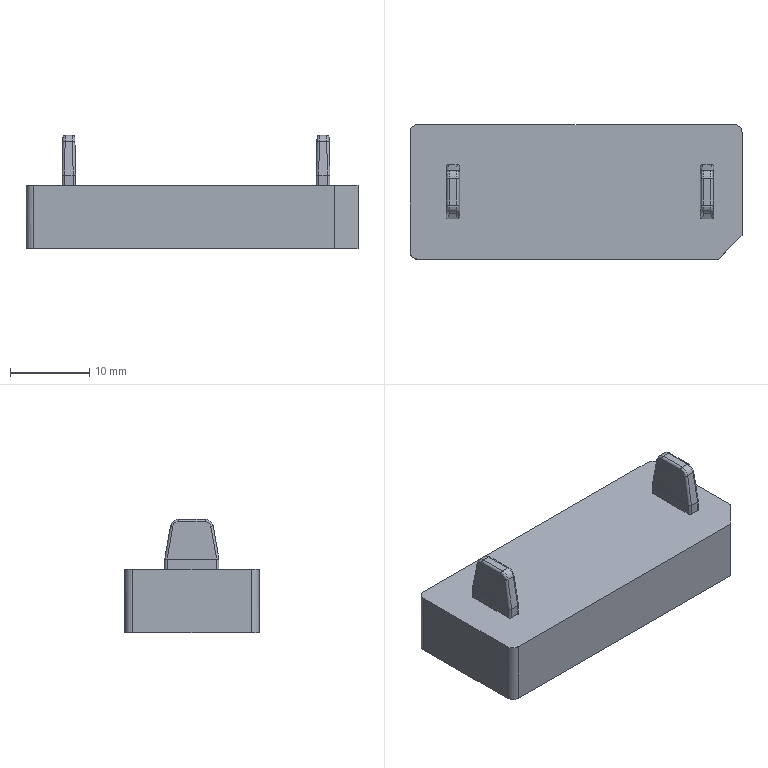NC program | PowerMill | posted by the shop | part box 42 x 17 x 14.346 mm
Lines 19164 to 20582 of 50900:
( TOOL ID   B4R0.5_2_1 )
( TOOL DIA. 4. TIP RAD .5 LENGTH 61.4 )
( Z = -6.519 )
T5 M6
T13
G91 G28 Z0
G0 G90 G54
M08
S18000 M3
X0 Y0 M8
G43 Z10.796 H5
X18.245 Y-3.811
Z.801
G1 Z-.399 F1200
X18.223 Y-3.743 F2000
X18.195 Y-3.678
X18.159 Y-3.616
X18.117 Y-3.558
X18.068 Y-3.506
X18.014 Y-3.459
X17.955 Y-3.419
X17.892 Y-3.386
X17.825 Y-3.359
X17.756 Y-3.341
X17.686 Y-3.33
X17.614 Y-3.327
X17.543 Y-3.332
X17.473 Y-3.345
X17.468 Y-3.346
X17.366 Y-3.372
X17.287 Y-3.386
X17.207 Y-3.398
X17.126 Y-3.404
X17.045 Y-3.406
X16.965
X16.575 Y-3.405
X16.186 Y-3.407
X16.072 Y-3.406
X15.958 Y-3.397
X15.845 Y-3.381
X15.733 Y-3.357
X15.623 Y-3.325
X15.516 Y-3.286
X15.412 Y-3.239
X15.321 Y-3.19
X15.232 Y-3.134
X15.142 Y-3.069
X15.05 Y-2.992
X14.972 Y-2.919
X14.899 Y-2.84
X14.83 Y-2.755
X14.766 Y-2.662
X14.706 Y-2.563
X14.652 Y-2.456
X14.603 Y-2.344
X14.56 Y-2.224
X14.536 Y-2.144
X14.518 Y-2.062
X14.502 Y-1.962
X14.489 Y-1.835
X14.481 Y-1.716
X14.478 Y-1.622
Y-1.538
X14.48 Y-.072
X14.481 Y.907
X14.479 Y1.531
X14.478 Y1.626
X14.479 Y1.722
X14.483 Y1.817
X14.49 Y1.913
X14.503 Y2.017
X14.524 Y2.125
X14.548 Y2.221
X14.577 Y2.312
X14.609 Y2.402
X14.653 Y2.503
X14.705 Y2.603
X14.765 Y2.701
X14.833 Y2.798
X14.902 Y2.884
X14.978 Y2.965
X15.061 Y3.043
X15.15 Y3.115
X15.244 Y3.181
X15.342 Y3.24
X15.444 Y3.293
X15.55 Y3.338
X15.658 Y3.376
X15.759 Y3.404
X15.865 Y3.425
X15.977 Y3.438
X16.096 Y3.445
X16.221 Y3.446
X17.104 Y3.443
X17.153 Y3.442
X17.203 Y3.438
X17.255 Y3.431
X17.323 Y3.419
X17.419 Y3.398
X17.495 Y3.378
X17.551 Y3.36
X17.598 Y3.343
X17.71 Y3.296
X17.807 Y3.248
X17.892 Y3.197
X17.973 Y3.142
X18.067 Y3.068
X18.154 Y2.99
X18.235 Y2.908
X18.308 Y2.822
X18.374 Y2.732
X18.433 Y2.639
X18.486 Y2.542
X18.538 Y2.43
X18.582 Y2.318
X18.618 Y2.205
X18.646 Y2.092
X18.663 Y1.991
X18.675 Y1.884
X18.681 Y1.759
Y1.599
X18.679 Y1.253
X18.68 Y.451
Y-.617
Y-1.551
X18.678 Y-1.721
X18.672 Y-1.851
X18.66 Y-1.963
X18.643 Y-2.064
X18.618 Y-2.164
X18.584 Y-2.27
X18.548 Y-2.367
X18.514 Y-2.448
X18.473 Y-2.527
X18.424 Y-2.613
X18.36 Y-2.71
X18.289 Y-2.805
X18.221 Y-2.885
X18.158 Y-2.951
X18.093 Y-3.01
X18.001 Y-3.084
X17.905 Y-3.15
X17.806 Y-3.208
X17.705 Y-3.259
X17.601 Y-3.303
X17.496 Y-3.338
X17.468 Y-3.346
X17.366 Y-3.373 Z-.4
X17.292 Y-3.387
X17.21 Y-3.4
X17.129 Y-3.407
X17.046 Y-3.41
X16.964
X16.5 Y-3.415 Z-.401
X16.159 Y-3.419 Z-.402
X16.036 Y-3.417
X15.923 Y-3.408 Z-.403
X15.817 Y-3.393
X15.717 Y-3.37
X15.62 Y-3.341
X15.506 Y-3.3
X15.404 Y-3.256
X15.325 Y-3.215 Z-.404
X15.248 Y-3.171
X15.175 Y-3.121
X15.099 Y-3.062
X15.032 Y-3.004
X14.967 Y-2.943 Z-.405
X14.905 Y-2.88
X14.836 Y-2.799
X14.769 Y-2.71
X14.707 Y-2.613 Z-.406
X14.65 Y-2.51
X14.601 Y-2.404
X14.56 Y-2.302 Z-.407
X14.525 Y-2.197
X14.495 Y-2.088
X14.474 Y-1.978 Z-.408
X14.46 Y-1.87
X14.453 Y-1.761
X14.45 Y-1.652 Z-.409
X14.443 Y-1.026 Z-.41
X14.437 Y-.195 Z-.413
X14.432 Y.722 Z-.415
X14.426 Y1.48 Z-.417
X14.425 Y1.605
Y1.732 Z-.418
X14.43 Y1.869
X14.44 Y1.986
X14.456 Y2.091 Z-.419
X14.478 Y2.195
X14.507 Y2.298
X14.546 Y2.411
X14.592 Y2.521
X14.646 Y2.63
X14.708 Y2.735
X14.777 Y2.837
X14.847 Y2.928
X14.924 Y3.014
X15.007 Y3.096 Z-.42
X15.097 Y3.173
X15.187 Y3.241
X15.282 Y3.302
X15.383 Y3.358
X15.489 Y3.408
X15.6 Y3.451 Z-.421
X15.703 Y3.484
X15.809 Y3.51
X15.92 Y3.528
X16.036 Y3.54 Z-.422
X16.156 Y3.544
X16.264
X16.515 Y3.545 Z-.423
X16.766 Y3.547 Z-.424
X17.017 Y3.548
X17.137 Y3.549 Z-.425
X17.223 Y3.545
X17.314 Y3.533
X17.411 Y3.513
X17.517 Y3.483 Z-.426
X17.619 Y3.448
X17.727 Y3.405 Z-.427
X17.829 Y3.355
X17.926 Y3.301
X18.016 Y3.24 Z-.428
X18.102 Y3.175
X18.184 Y3.104
X18.263 Y3.028 Z-.429
X18.337 Y2.947
X18.407 Y2.858 Z-.43
X18.471 Y2.766
X18.528 Y2.669 Z-.431
X18.581 Y2.57
X18.624 Y2.474
X18.663 Y2.369 Z-.432
X18.698 Y2.255
X18.728 Y2.131
X18.751 Y2.001
X18.765 Y1.877 Z-.433
X18.772 Y1.761
X18.773 Y1.652
X18.781 Y-.205 Z-.438
X18.79 Y-1.402 Z-.441
X18.792 Y-1.554
X18.79 Y-1.713 Z-.442
X18.781 Y-1.86
X18.765 Y-1.997
X18.744 Y-2.125 Z-.443
X18.715 Y-2.245
X18.681 Y-2.359
X18.641 Y-2.467
X18.599 Y-2.56 Z-.444
X18.549 Y-2.656
X18.488 Y-2.76
X18.417 Y-2.865 Z-.445
X18.345 Y-2.959
X18.275 Y-3.04
X18.204 Y-3.111
X18.129 Y-3.177 Z-.446
X18.035 Y-3.252
X17.938 Y-3.318
X17.839 Y-3.377
X17.736 Y-3.428 Z-.447
X17.631 Y-3.472
X17.523 Y-3.51
X17.517 Y-3.512
X17.393 Y-3.544
X17.27 Y-3.567 Z-.448
X17.149 Y-3.582
X17.031 Y-3.59
X16.912 Z-.449
X16.504 Y-3.591
X16.159 Y-3.595 Z-.45
X16.055 Y-3.594 Z-.451
X15.951 Y-3.587
X15.846 Y-3.573
X15.737 Y-3.55
X15.632 Y-3.521 Z-.452
X15.531 Y-3.488
X15.424 Y-3.445
X15.324 Y-3.397
X15.23 Y-3.344 Z-.453
X15.142 Y-3.285
X15.056 Y-3.222
X14.969 Y-3.149
X14.892 Y-3.076 Z-.454
X14.82 Y-2.998
X14.753 Y-2.917
X14.681 Y-2.817
X14.615 Y-2.713 Z-.455
X14.556 Y-2.606
X14.505 Y-2.494
X14.46 Y-2.38 Z-.456
X14.423 Y-2.263
X14.391 Y-2.137
X14.367 Y-2.011 Z-.457
X14.351 Y-1.886
X14.343 Y-1.761
X14.342 Y-1.637
X14.337 Y-.269 Z-.461
X14.333 Y.812 Z-.463
X14.327 Y1.545 Z-.465
X14.326 Y1.649
X14.327 Y1.752
X14.331 Y1.856 Z-.466
X14.34 Y1.959
X14.354 Y2.07
X14.373 Y2.172
X14.397 Y2.272 Z-.467
X14.424 Y2.372
X14.463 Y2.488
X14.509 Y2.601
X14.561 Y2.709 Z-.468
X14.622 Y2.817
X14.689 Y2.919
X14.76 Y3.015
X14.837 Y3.105 Z-.469
X14.907 Y3.178
X14.987 Y3.252
X15.078 Y3.327 Z-.47
X15.177 Y3.398
X15.275 Y3.459
X15.369 Y3.51
X15.46 Y3.551 Z-.471
X15.546 Y3.583
X15.63 Y3.612
X15.716 Y3.636
X15.841 Y3.665
X15.933 Y3.68 Z-.472
X16.036 Y3.688
X16.157 Y3.691
X16.316 Z-.473
X16.772 Y3.694 Z-.474
X16.977 Y3.697
X17.1 Y3.696
X17.217 Y3.687 Z-.475
X17.329 Y3.672
X17.437 Y3.649
X17.542 Y3.62
X17.658 Y3.579 Z-.476
X17.769 Y3.533
X17.874 Y3.481
X17.975 Y3.422 Z-.477
X18.071 Y3.356
X18.163 Y3.284
X18.25 Y3.206
X18.333 Y3.121 Z-.478
X18.412 Y3.029
X18.485 Y2.933
X18.553 Y2.831 Z-.479
X18.614 Y2.723
X18.669 Y2.611
X18.717 Y2.494
X18.759 Y2.373 Z-.48
X18.794 Y2.248
X18.821 Y2.119
X18.841 Y1.987 Z-.481
X18.853 Y1.852
X18.858 Y1.716
Y1.578 Z-.482
X18.862 Y.382 Z-.484
X18.865 Y-.57 Z-.487
X18.869 Y-1.524 Z-.489
Y-1.717
X18.865 Y-1.846 Z-.49
X18.853 Y-1.975
X18.833 Y-2.104
X18.805 Y-2.232
X18.769 Y-2.359 Z-.491
X18.726 Y-2.484
X18.674 Y-2.608
X18.621 Y-2.717 Z-.492
X18.561 Y-2.823
X18.494 Y-2.925
X18.42 Y-3.023 Z-.493
X18.34 Y-3.117
X18.253 Y-3.205
X18.176 Y-3.276
X18.091 Y-3.344 Z-.494
X17.994 Y-3.412
X17.891 Y-3.475
X17.788 Y-3.529
X17.689 Y-3.573 Z-.495
X17.596 Y-3.608
X17.551 Y-3.621
X17.441 Y-3.654
X17.361 Y-3.674 Z-.496
X17.281 Y-3.688
X17.168 Y-3.701
X17.045 Y-3.707
X16.908 Y-3.708 Z-.497
X16.475 Y-3.71 Z-.498
X16.159 Y-3.713
X16.042 Y-3.71 Z-.499
X15.923 Y-3.701
X15.807 Y-3.684
X15.753 Y-3.673
X15.699 Y-3.659
X15.642 Y-3.642
X15.568 Y-3.619 Z-.5
X15.464 Y-3.581
X15.393 Y-3.553
X15.341 Y-3.528
X15.291 Y-3.503
X15.185 Y-3.441 Z-.501
X15.084 Y-3.374
X14.989 Y-3.3
X14.9 Y-3.222
X14.817 Y-3.138 Z-.502
X14.738 Y-3.048
X14.663 Y-2.95
X14.594 Y-2.846
X14.529 Y-2.736 Z-.503
X14.471 Y-2.621
X14.421 Y-2.503
X14.378 Y-2.384 Z-.504
X14.343 Y-2.262
X14.313 Y-2.131
X14.29 Y-1.998 Z-.505
X14.276 Y-1.869
X14.27 Y-1.745
X14.269 Y-1.621
X14.265 Y-.061 Z-.509
X14.262 Y.996 Z-.511
X14.258 Y1.593 Z-.513
X14.259 Y1.757
X14.267 Y1.908
X14.281 Y2.048 Z-.514
X14.301 Y2.178
X14.329 Y2.303
X14.363 Y2.424 Z-.515
X14.406 Y2.549
X14.455 Y2.669
X14.511 Y2.784 Z-.516
X14.573 Y2.893
X14.642 Y2.999
X14.717 Y3.099
X14.797 Y3.194 Z-.517
X14.882 Y3.282
X14.973 Y3.364
X15.067 Y3.439
X15.165 Y3.507 Z-.518
X15.267 Y3.568
X15.372 Y3.621
X15.481 Y3.668 Z-.519
X15.596 Y3.709
X15.714 Y3.742
X15.833 Y3.767
X15.953 Y3.785 Z-.52
X16.075 Y3.795
X16.196 Y3.797
X16.755 Y3.798 Z-.521
X16.918 Y3.799 Z-.522
X17.065 Y3.8
X17.179 Y3.795
X17.28 Y3.784 Z-.523
X17.322 Y3.777
X17.365 Y3.768
X17.417 Y3.757
X17.499 Y3.737
X17.55 Y3.723
X17.591 Y3.711
X17.631 Y3.695 Z-.524
X17.715 Y3.662
X17.798 Y3.628
X17.879 Y3.588
X17.983 Y3.528
X18.083 Y3.462 Z-.525
X18.179 Y3.388
X18.27 Y3.308
X18.357 Y3.221
X18.439 Y3.128 Z-.526
X18.515 Y3.029
X18.585 Y2.925
X18.65 Y2.816 Z-.527
X18.707 Y2.703
X18.758 Y2.585
X18.804 Y2.456 Z-.528
X18.843 Y2.325
X18.874 Y2.194
X18.897 Y2.064
X18.911 Y1.934 Z-.529
X18.918 Y1.806
X18.919 Y1.679
X18.923 Y.67 Z-.532
X18.927 Y-.867 Z-.535
X18.928 Y-1.714 Z-.537
X18.923 Y-1.852
X18.911 Y-1.988 Z-.538
X18.892 Y-2.123
X18.864 Y-2.256
X18.829 Y-2.387 Z-.539
X18.786 Y-2.514
X18.737 Y-2.636
X18.682 Y-2.753
X18.619 Y-2.866 Z-.54
X18.551 Y-2.974
X18.476 Y-3.077
X18.404 Y-3.165 Z-.541
X18.323 Y-3.251
X18.234 Y-3.335
X18.137 Y-3.415
X18.037 Y-3.488 Z-.542
X17.935 Y-3.552
X17.834 Y-3.608
X17.735 Y-3.654
X17.638 Y-3.691 Z-.543
X17.578 Y-3.709
X17.47 Y-3.74
X17.357 Y-3.767
X17.241 Y-3.786 Z-.544
X17.13 Y-3.798
X17.019 Y-3.803
X16.908
X16.408 Y-3.804 Z-.546
X16.16 Y-3.807
X16.046 Y-3.805
X15.93 Y-3.795 Z-.547
X15.813 Y-3.777
X15.695 Y-3.751
X15.574 Y-3.716
X15.462 Y-3.677 Z-.548
X15.352 Y-3.63
X15.245 Y-3.576
X15.143 Y-3.516
X15.045 Y-3.448 Z-.549
X14.95 Y-3.373
X14.859 Y-3.292
X14.773 Y-3.203 Z-.55
X14.691 Y-3.109
X14.615 Y-3.008
X14.545 Y-2.901
X14.48 Y-2.79 Z-.551
X14.422 Y-2.673
X14.371 Y-2.553
X14.331 Y-2.438
X14.296 Y-2.318 Z-.552
X14.265 Y-2.186
X14.24 Y-2.046
X14.224 Y-1.91 Z-.553
X14.216 Y-1.783
X14.214 Y-1.658
X14.21 Y.297 Z-.558
X14.206 Y1.717 Z-.561
X14.209 Y1.862
X14.22 Y2.005
X14.239 Y2.144 Z-.562
X14.266 Y2.281
X14.299 Y2.413
X14.339 Y2.542 Z-.563
X14.387 Y2.666
X14.441 Y2.785
X14.501 Y2.9 Z-.564
X14.568 Y3.01
X14.64 Y3.114
X14.719 Y3.213
X14.802 Y3.305 Z-.565
X14.89 Y3.391
X14.983 Y3.471
X15.071 Y3.537
X15.163 Y3.599 Z-.566
X15.264 Y3.657
X15.358 Y3.706
X15.424 Y3.735
X15.491 Y3.761
X15.573 Y3.789 Z-.567
X15.678 Y3.821
X15.748 Y3.839
X15.819 Y3.854
X15.89 Y3.865
X16.011 Y3.877 Z-.568
X16.14 Y3.882
X16.279 Y3.883
X16.852 Y3.885 Z-.57
X16.977
X17.059
X17.167 Y3.882
X17.255 Y3.873
X17.336 Y3.859 Z-.571
X17.44 Y3.838
X17.543 Y3.811
X17.66 Y3.772
X17.774 Y3.726 Z-.572
X17.884 Y3.673
X17.991 Y3.614
X18.093 Y3.547
X18.191 Y3.473 Z-.573
X18.283 Y3.395
X18.369 Y3.312
X18.451 Y3.221 Z-.574
X18.529 Y3.123
X18.602 Y3.019
X18.669 Y2.909
X18.73 Y2.793 Z-.575
X18.785 Y2.673
X18.832 Y2.549
X18.873 Y2.423 Z-.576
X18.907 Y2.292
X18.933 Y2.158
X18.953 Y2.02
X18.965 Y1.879 Z-.577
X18.97 Y1.732
Y1.583
X18.972 Y.357 Z-.58
X18.974 Y-.867 Z-.583
X18.978 Y-1.582 Z-.584
X18.976 Y-1.75 Z-.585
X18.967 Y-1.907
X18.951 Y-2.054 Z-.586
X18.928 Y-2.194
X18.899 Y-2.326
X18.863 Y-2.454
X18.819 Y-2.582 Z-.587
X18.768 Y-2.705
X18.711 Y-2.824
X18.647 Y-2.937 Z-.588
X18.578 Y-3.046
X18.51 Y-3.138
X18.437 Y-3.226
X18.351 Y-3.318 Z-.589
X18.255 Y-3.41
X18.163 Y-3.489
X18.119 Y-3.523
X18.081 Y-3.55
X18.04 Y-3.576 Z-.59
X17.987 Y-3.608
X17.915 Y-3.648
X17.814 Y-3.7
X17.743 Y-3.733
X17.687 Y-3.756
X17.643 Y-3.772 Z-.591
X17.599 Y-3.784
X17.495 Y-3.815
X17.389 Y-3.841
X17.279 Y-3.86
X17.17 Y-3.872 Z-.592
X17.062 Y-3.878
X16.953 Y-3.88
X16.432 Y-3.882 Z-.593
X16.16 Y-3.883 Z-.594
X16.076
X15.994 Y-3.879
X15.9 Y-3.868
X15.832 Y-3.859 Z-.595
X15.803 Y-3.854
X15.772 Y-3.848
X15.723 Y-3.837
X15.694 Y-3.83
X15.666 Y-3.823
X15.566 Y-3.794
X15.488 Y-3.769
X15.375 Y-3.723 Z-.596
X15.266 Y-3.67
X15.159 Y-3.61
X15.057 Y-3.543
X14.958 Y-3.469 Z-.597
X14.864 Y-3.389
X14.775 Y-3.302
X14.692 Y-3.21 Z-.598
X14.614 Y-3.111
X14.542 Y-3.007
X14.475 Y-2.897
X14.413 Y-2.781 Z-.599
X14.359 Y-2.66
X14.31 Y-2.535
X14.268 Y-2.403 Z-.6
X14.233 Y-2.268
X14.205 Y-2.132
X14.186 Y-1.993
X14.174 Y-1.852 Z-.601
X14.17 Y-1.709
X14.168 Y-.346 Z-.604
X14.165 Y.94 Z-.607
X14.162 Y1.593 Z-.608
X14.164 Y1.775 Z-.609
X14.172 Y1.937
X14.186 Y2.084
X14.207 Y2.221 Z-.61
X14.234 Y2.351
X14.27 Y2.486
X14.313 Y2.616 Z-.611
X14.363 Y2.741
X14.42 Y2.862
X14.482 Y2.978
X14.55 Y3.087 Z-.612
X14.624 Y3.191
X14.703 Y3.288
X14.787 Y3.38 Z-.613
X14.876 Y3.465
X14.969 Y3.543
X15.067 Y3.614
X15.173 Y3.684 Z-.614
X15.276 Y3.742
X15.376 Y3.791
X15.459 Y3.825
X15.543 Y3.856
X15.63 Y3.882 Z-.615
X15.689 Y3.898
X15.748 Y3.914
X15.808 Y3.927
X15.869 Y3.935
X15.969 Y3.948
X16.053 Y3.954 Z-.616
X16.16 Y3.955
X16.739 Y3.957 Z-.617
X16.979 Y3.958 Z-.618
X17.103 Y3.955
X17.227 Y3.946
X17.35 Y3.929
X17.46 Y3.907 Z-.619
X17.549 Y3.885
X17.636 Y3.857
X17.729 Y3.821
X17.837 Y3.774 Z-.62
X17.944 Y3.72
X18.032 Y3.668
X18.108 Y3.617
X18.215 Y3.536 Z-.621
X18.307 Y3.457
X18.389 Y3.378
X18.475 Y3.284
X18.553 Y3.187 Z-.622
X18.625 Y3.084
X18.693 Y2.975
X18.754 Y2.86
X18.81 Y2.74 Z-.623
X18.859 Y2.615
X18.902 Y2.485
X18.938 Y2.351 Z-.624
X18.967 Y2.211
X18.988 Y2.067
X19.003 Y1.919 Z-.625
X19.009 Y1.768
X19.01 Y1.613
X19.014 Y-.465 Z-.63
Y-1.715 Z-.633
X19.01 Y-1.863
X18.998 Y-2.009
X18.978 Y-2.152 Z-.634
X18.951 Y-2.292
X18.917 Y-2.428
X18.876 Y-2.561
X18.827 Y-2.688 Z-.635
X18.773 Y-2.812
X18.711 Y-2.93
X18.647 Y-3.038 Z-.636
X18.577 Y-3.142
X18.499 Y-3.243
X18.413 Y-3.34
X18.328 Y-3.425 Z-.637
X18.235 Y-3.507
X18.137 Y-3.583
X18.033 Y-3.654 Z-.638
X17.927 Y-3.716
X17.818 Y-3.771
X17.709 Y-3.817
X17.618 Y-3.85 Z-.639
X17.514 Y-3.88
X17.41 Y-3.906
X17.301 Y-3.927
X17.194 Y-3.941
X17.086 Y-3.948 Z-.64
X16.979 Y-3.95
X16.871 Y-3.949
X16.336 Y-3.95 Z-.641
X16.16 Y-3.952 Z-.642
X16.039 Y-3.95
X15.917 Y-3.939
X15.796 Y-3.921
X15.674 Y-3.895 Z-.643
X15.554 Y-3.86
X15.437 Y-3.819
X15.323 Y-3.77 Z-.644
X15.213 Y-3.714
X15.107 Y-3.651
X15.007 Y-3.582
X14.911 Y-3.508 Z-.645
X14.817 Y-3.424
X14.728 Y-3.334
X14.645 Y-3.239
X14.569 Y-3.139 Z-.646
X14.499 Y-3.034
X14.432 Y-2.921
X14.371 Y-2.802 Z-.647
X14.317 Y-2.679
X14.27 Y-2.551
X14.229 Y-2.42
X14.196 Y-2.285 Z-.648
X14.17 Y-2.148
X14.15 Y-2.
X14.138 Y-1.853 Z-.649
X14.134 Y-1.707
X14.131 Y-.191 Z-.652
X14.13 Y1.064 Z-.655
X14.127 Y1.593 Z-.656
X14.128 Y1.723
X14.131 Y1.854 Z-.657
X14.139 Y1.984
X14.155 Y2.122
X14.175 Y2.251
X14.201 Y2.376 Z-.658
X14.235 Y2.511
X14.276 Y2.64
X14.323 Y2.761 Z-.659
X14.376 Y2.878
X14.439 Y2.998
X14.507 Y3.111
X14.579 Y3.217 Z-.66
X14.657 Y3.315
X14.738 Y3.407
X14.827 Y3.496 Z-.661
X14.922 Y3.579
X15.019 Y3.655
X15.117 Y3.721
X15.215 Y3.779 Z-.662
X15.299 Y3.824
X15.386 Y3.863
X15.479 Y3.9
X15.59 Y3.937
X15.686 Y3.963 Z-.663
X15.766 Y3.98
X15.87 Y4.
X15.949 Y4.011
X16.021 Y4.014
X16.365 Y4.019 Z-.664
X16.704 Y4.02 Z-.665
X16.892 Y4.022
X17.05 Y4.021 Z-.666
X17.176 Y4.015
X17.285 Y4.004
X17.391 Y3.986
X17.513 Y3.958 Z-.667
X17.633 Y3.923
X17.748 Y3.881
X17.86 Y3.831
X17.968 Y3.775 Z-.668
X18.073 Y3.711
X18.174 Y3.641
X18.271 Y3.563
X18.364 Y3.479 Z-.669
X18.451 Y3.389
X18.533 Y3.294
X18.61 Y3.193 Z-.67
X18.681 Y3.087
X18.746 Y2.975
X18.805 Y2.857
X18.859 Y2.734 Z-.671
X18.905 Y2.605
X18.946 Y2.472
X18.98 Y2.333 Z-.672
X19.006 Y2.189
X19.026 Y2.04
X19.038 Y1.887 Z-.673
X19.043 Y1.73
Y1.57
X19.044 Y.166 Z-.676
X19.046 Y-1.582 Z-.68
Y-1.695
X19.043 Y-1.807 Z-.681
X19.038 Y-1.92
X19.029 Y-2.032
X19.014 Y-2.144
X18.992 Y-2.265 Z-.682
X18.967 Y-2.375
X18.938 Y-2.484
X18.905 Y-2.591
X18.86 Y-2.717 Z-.683
X18.807 Y-2.839
X18.748 Y-2.956
X18.682 Y-3.069
X18.611 Y-3.176 Z-.684
X18.533 Y-3.278
X18.45 Y-3.375
X18.36 Y-3.466
X18.266 Y-3.551 Z-.685
X18.168 Y-3.629
X18.065 Y-3.7
X17.96 Y-3.764 Z-.686
X17.851 Y-3.82
X17.741 Y-3.868
X17.639 Y-3.905
X17.574 Y-3.926
X17.509 Y-3.944 Z-.687
X17.422 Y-3.966
X17.317 Y-3.987
X17.239 Y-3.998
X17.172 Y-4.005
X17.104 Y-4.007
X16.603 Y-4.012 Z-.689
X16.251
X15.996 Y-4.007 Z-.69
X15.905 Y-4.
X15.807 Y-3.985
X15.698 Y-3.962
X15.573 Y-3.927 Z-.691
X15.469 Y-3.893
X15.366 Y-3.853
X15.262 Y-3.804
X15.156 Y-3.746 Z-.692
X15.048 Y-3.678
X14.949 Y-3.607
X14.855 Y-3.529 Z-.693
X14.764 Y-3.444
X14.678 Y-3.353
X14.597 Y-3.255
X14.521 Y-3.15 Z-.694
X14.45 Y-3.04
X14.385 Y-2.925
X14.327 Y-2.804
X14.275 Y-2.679 Z-.695
X14.23 Y-2.549
X14.192 Y-2.414
X14.16 Y-2.273 Z-.696
X14.135 Y-2.127
X14.117 Y-1.978
X14.107 Y-1.825 Z-.697
X14.105 Y-1.67
X14.101 Y.341 Z-.701
X14.099 Y1.714 Z-.704
X14.102 Y1.856
X14.112 Y2.01 Z-.705
X14.13 Y2.167
X14.155 Y2.315
X14.184 Y2.45 Z-.706
X14.218 Y2.575
X14.262 Y2.706
X14.312 Y2.833 Z-.707
X14.368 Y2.954
X14.431 Y3.07
X14.5 Y3.181
X14.575 Y3.286 Z-.708
X14.656 Y3.386
X14.742 Y3.481
X14.834 Y3.57
X14.926 Y3.648 Z-.709
X15.023 Y3.722
X15.128 Y3.79
X15.218 Y3.842
X15.31 Y3.889 Z-.71
X15.405 Y3.931
X15.502 Y3.967
X15.596 Y3.998
X15.712 Y4.03 Z-.711
X15.823 Y4.052
X15.926 Y4.066
X16.024 Y4.072
X16.212 Y4.076 Z-.712
X16.399
X16.587
X16.978 Y4.077 Z-.713
X17.11 Y4.075 Z-.714
X17.238 Y4.065
X17.362 Y4.048
X17.483 Y4.023
X17.602 Y3.991 Z-.715
X17.718 Y3.951
X17.831 Y3.904
X17.94 Y3.85
X18.046 Y3.789 Z-.716
X18.15 Y3.72
X18.251 Y3.643
X18.349 Y3.559
X18.44 Y3.469 Z-.717
X18.525 Y3.376
X18.601 Y3.28
X18.675 Y3.174 Z-.718
X18.743 Y3.063
X18.805 Y2.947
X18.861 Y2.826
X18.91 Y2.699 Z-.719
X18.953 Y2.566
X18.99 Y2.428
X19.02 Y2.284 Z-.72
X19.043 Y2.135
X19.059 Y1.98
X19.068 Y1.82 Z-.721
X19.07 Y1.654
X19.072 Y-.697 Z-.726
X19.073 Y-1.717 Z-.728
X19.069 Y-1.873
X19.057 Y-2.027 Z-.729
X19.038 Y-2.177
X19.011 Y-2.325
X18.977 Y-2.469 Z-.73
X18.935 Y-2.609
X18.891 Y-2.735
X18.839 Y-2.858 Z-.731
X18.781 Y-2.977
X18.715 Y-3.092
X18.643 Y-3.202
X18.565 Y-3.307 Z-.732
X18.481 Y-3.408
X18.397 Y-3.496
X18.307 Y-3.579 Z-.733
X18.21 Y-3.659
X18.107 Y-3.732
X18.001 Y-3.798
X17.893 Y-3.856 Z-.734
X17.785 Y-3.906
X17.678 Y-3.947
X17.657 Y-3.954
X17.59 Y-3.978
X17.511 Y-4.
X17.406 Y-4.023 Z-.735
X17.297 Y-4.043
X17.212 Y-4.055
X17.113 Y-4.061
X16.982 Y-4.063 Z-.736
X16.446 Y-4.064 Z-.737
X16.158 Y-4.065
X16.032 Y-4.062 Z-.738
X15.906 Y-4.051
X15.78 Y-4.032
X15.656 Y-4.005
X15.537 Y-3.972 Z-.739
X15.421 Y-3.931
X15.307 Y-3.882
X15.197 Y-3.827
X15.09 Y-3.764 Z-.74
X14.987 Y-3.694
X14.888 Y-3.618
X14.793 Y-3.535
X14.703 Y-3.445 Z-.741
X14.618 Y-3.349
X14.539 Y-3.247
X14.465 Y-3.14 Z-.742
X14.398 Y-3.027
X14.337 Y-2.91
X14.28 Y-2.785
X14.231 Y-2.656 Z-.743
X14.188 Y-2.523
X14.153 Y-2.385
X14.124 Y-2.242 Z-.744
X14.102 Y-2.094
X14.087 Y-1.941
X14.08 Y-1.783 Z-.745
X14.079 Y-1.62
X14.078 Y.52 Z-.749
X14.075 Y1.593 Z-.752
X14.077 Y1.792
X14.086 Y1.969
X14.1 Y2.132 Z-.753
X14.121 Y2.282
X14.148 Y2.423
X14.18 Y2.556 Z-.754
X14.22 Y2.684
X14.266 Y2.808
X14.32 Y2.934 Z-.755
X14.379 Y3.052
X14.442 Y3.162
X14.509 Y3.264
X14.583 Y3.363 Z-.756
X14.667 Y3.463
X14.752 Y3.554
X14.839 Y3.636
X14.927 Y3.709 Z-.757
X15.019 Y3.775
X15.13 Y3.847
X15.24 Y3.909
X15.349 Y3.963 Z-.758
X15.413 Y3.99
X15.478 Y4.013
X15.543 Y4.034
X15.621 Y4.056
X15.727 Y4.083
X15.826 Y4.103 Z-.759
X15.902 Y4.115
X15.97 Y4.122
X16.039 Y4.124
X16.423 Y4.128 Z-.76
X16.704 Z-.761
X16.901 Y4.13
X17.062 Y4.129
X17.19 Y4.123 Z-.762
X17.305 Y4.111
X17.38 Y4.098
X17.455 Y4.081
X17.539 Y4.06
X17.637 Y4.032 Z-.763
X17.709 Y4.008
X17.78 Y3.981
X17.895 Y3.927
X18.008 Y3.866
X18.11 Y3.805 Z-.764
X18.202 Y3.742
X18.293 Y3.669
X18.383 Y3.588
X18.472 Y3.498 Z-.765
X18.559 Y3.398
X18.635 Y3.3
X18.706 Y3.197
X18.772 Y3.086 Z-.766
X18.832 Y2.969
X18.888 Y2.845
X18.937 Y2.717 Z-.767
X18.979 Y2.585
X19.014 Y2.448
X19.043 Y2.304
X19.065 Y2.154 Z-.768
X19.081 Y1.995
X19.09 Y1.829
X19.091 Y1.654 Z-.769
X19.093 Y-1.032 Z-.774
Y-1.714 Z-.776
X19.09 Y-1.871
X19.078 Y-2.031 Z-.777
X19.06 Y-2.188
X19.034 Y-2.339
X19.003 Y-2.481 Z-.778
X18.966 Y-2.613
X18.923 Y-2.738
X18.872 Y-2.865
X18.814 Y-2.987 Z-.779
X18.75 Y-3.103
X18.68 Y-3.215
X18.605 Y-3.32 Z-.78
X18.523 Y-3.42
X18.437 Y-3.514
X18.345 Y-3.601
X18.249 Y-3.683 Z-.781
X18.147 Y-3.758
X18.041 Y-3.828
X17.937 Y-3.886
X17.828 Y-3.939 Z-.782
X17.713 Y-3.986
X17.673 Y-4.
X17.581 Y-4.029
X17.488 Y-4.055
X17.394 Y-4.075 Z-.783
X17.269 Y-4.094
X17.14 Y-4.106
X17.002 Y-4.111
X16.857 Y-4.112 Z-.784
X16.432 Z-.785
X16.16 Y-4.113
X16.074
X15.989 Y-4.109
X15.891 Y-4.097 Z-.786
X15.83 Y-4.09
X15.769 Y-4.08
X15.709 Y-4.067
X15.623 Y-4.047
X15.563 Y-4.03
X15.504 Y-4.012 Z-.787
X15.371 Y-3.96
X15.261 Y-3.911
X15.163 Y-3.86
X15.056 Y-3.795 Z-.788
X14.953 Y-3.724
X14.854 Y-3.645
X14.76 Y-3.56
X14.67 Y-3.468 Z-.789
X14.586 Y-3.371
X14.507 Y-3.267
X14.434 Y-3.159
X14.368 Y-3.045 Z-.79
X14.308 Y-2.928
X14.255 Y-2.805
X14.208 Y-2.677 Z-.791
X14.167 Y-2.543
X14.132 Y-2.403
X14.104 Y-2.257
X14.083 Y-2.104 Z-.792
X14.069 Y-1.945
X14.062 Y-1.778
X14.061 Y-1.605 Z-.793
X14.058 Y1.032 Z-.798
Y1.716 Z-.8
X14.061 Y1.885
X14.07 Y2.049
X14.086 Y2.203 Z-.801
X14.108 Y2.348
X14.137 Y2.485
X14.172 Y2.619 Z-.802
X14.211 Y2.744
X14.256 Y2.866
X14.31 Y2.987
X14.369 Y3.103 Z-.803
X14.433 Y3.213
X14.505 Y3.321
X14.583 Y3.424
X14.667 Y3.521 Z-.804
X14.756 Y3.613
X14.851 Y3.699
X14.95 Y3.778 Z-.805
X15.054 Y3.851
X15.162 Y3.916
X15.269 Y3.972
X15.381 Y4.023 Z-.806
X15.498 Y4.066
X15.62 Y4.104
X15.745 Y4.133
X15.871 Y4.155 Z-.807
X15.996 Y4.168
X16.118 Y4.174
X16.238 Y4.173
X16.685 Z-.808
X16.976 Y4.176 Z-.809
X17.097 Y4.175
X17.223 Y4.165
X17.351 Y4.148 Z-.81
X17.478 Y4.122
X17.602 Y4.089
X17.721 Y4.05 Z-.811
X17.834 Y4.005
X17.939 Y3.954
X18.04 Y3.898
X18.146 Y3.831 Z-.812
X18.247 Y3.758
X18.342 Y3.679
X18.432 Y3.594
X18.517 Y3.504 Z-.813
X18.598 Y3.408
X18.676 Y3.303
X18.748 Y3.193
X18.813 Y3.077 Z-.814
X18.872 Y2.958
X18.924 Y2.834
X18.969 Y2.706
X19.008 Y2.573 Z-.815
X19.041 Y2.432
X19.068 Y2.284
X19.088 Y2.128 Z-.816
X19.101 Y1.962
X19.108 Y1.787
Y1.598 Z-.817
X19.11 Y-1.139 Z-.823
X19.111 Y-1.714 Z-.824
X19.107 Y-1.886
X19.096 Y-2.05
X19.077 Y-2.207 Z-.825
X19.052 Y-2.359
X19.02 Y-2.504
X18.982 Y-2.643 Z-.826
X18.937 Y-2.776
X18.888 Y-2.898
X18.833 Y-3.018 Z-.827
X18.769 Y-3.134
X18.699 Y-3.247
X18.621 Y-3.356
X18.544 Y-3.453 Z-.828
X18.458 Y-3.546
X18.366 Y-3.635
X18.269 Y-3.718
X18.167 Y-3.794 Z-.829
X18.063 Y-3.863
X17.956 Y-3.924
X17.849 Y-3.976
X17.741 Y-4.02 Z-.83
X17.687 Y-4.039
X17.604 Y-4.069
X17.519 Y-4.092
X17.434 Y-4.112
X17.317 Y-4.133 Z-.831
X17.193 Y-4.147
X17.06 Y-4.155
X16.914 Y-4.156
X16.432 Y-4.157 Z-.832
X16.16 Z-.833
X16.074
X15.989 Y-4.153
X15.893 Y-4.142 Z-.834
X15.833 Y-4.134
X15.786 Y-4.127
X15.74 Y-4.117
X15.686 Y-4.105
X15.613 Y-4.086
X15.516 Y-4.059
X15.451 Y-4.039
X15.402 Y-4.021 Z-.835
X15.359 Y-4.003
X15.316 Y-3.983
X15.19 Y-3.92
X15.087 Y-3.863
X14.998 Y-3.805
X14.896 Y-3.729 Z-.836
X14.798 Y-3.646
X14.706 Y-3.558
X14.619 Y-3.464 Z-.837
X14.537 Y-3.364
X14.461 Y-3.259
X14.391 Y-3.149
X14.328 Y-3.033 Z-.838
X14.27 Y-2.912
X14.219 Y-2.786
X14.175 Y-2.655
X14.139 Y-2.527 Z-.839
X14.106 Y-2.381
X14.081 Y-2.233
X14.062 Y-2.079 Z-.84
X14.05 Y-1.917
X14.046 Y-1.747
X14.045 Y-1.57 Z-.841
X14.044 Y1.593 Z-.847
Y1.711
X14.046 Y1.829 Z-.848
X14.049 Y1.947
X14.055 Y2.065
X14.066 Y2.185
X14.084 Y2.321 Z-.849
X14.107 Y2.446
X14.133 Y2.56
X14.164 Y2.674 Z-.85
X14.199 Y2.786
X14.245 Y2.909
X14.297 Y3.026
X14.359 Y3.146 Z-.851
X14.427 Y3.261
X14.501 Y3.37
X14.58 Y3.473
X14.665 Y3.57 Z-.852
X14.754 Y3.661
X14.848 Y3.745
X14.947 Y3.823
X15.051 Y3.895 Z-.853
X15.159 Y3.96
X15.271 Y4.018
X15.387 Y4.069
X15.505 Y4.113 Z-.854
X15.626 Y4.149
X15.748 Y4.177
X15.872 Y4.197
X15.997 Y4.209 Z-.855
X16.088 Y4.213
X16.179 Y4.215
X16.27 Y4.217
X16.367 Z-.856
X16.492 Y4.218
X16.673
X16.791
X16.883 Y4.217 Z-.857
X16.974 Y4.216
X17.065 Y4.215
X17.156 Y4.212
X17.268 Y4.203
X17.384 Y4.185 Z-.858
X17.504 Y4.159
X17.626 Y4.126
X17.744 Y4.085
X17.86 Y4.037 Z-.859
X17.972 Y3.981
X18.081 Y3.919
X18.186 Y3.849
X18.287 Y3.773 Z-.86
X18.383 Y3.69
X18.475 Y3.601
X18.561 Y3.506
X18.642 Y3.404 Z-.861
X18.717 Y3.297
X18.787 Y3.185
X18.85 Y3.068 Z-.862
X18.906 Y2.946
X18.956 Y2.82
X18.999 Y2.69
X19.035 Y2.555 Z-.863
X19.065 Y2.413
X19.089 Y2.263
X19.106 Y2.103 Z-.864
X19.117 Y1.931
X19.122 Y1.743
Y1.534 Z-.865
Y-1.717 Z-.872
X19.119 Y-1.897
X19.109 Y-2.065
X19.092 Y-2.224 Z-.873
X19.069 Y-2.374
X19.04 Y-2.516
X19.004 Y-2.652
X18.962 Y-2.782 Z-.874
X18.913 Y-2.906
X18.859 Y-3.026
X18.798 Y-3.141 Z-.875
X18.73 Y-3.252
X18.66 Y-3.356
X18.582 Y-3.456
X18.498 Y-3.552 Z-.876
X18.407 Y-3.644
X18.311 Y-3.729
X18.211 Y-3.808
X18.107 Y-3.879 Z-.877
X18.001 Y-3.943
X17.894 Y-3.998
X17.787 Y-4.045
X17.7 Y-4.076 Z-.878
X17.609 Y-4.108
X17.507 Y-4.136
X17.387 Y-4.161
X17.273 Y-4.179
X17.151 Y-4.19 Z-.879
X17.013 Y-4.195
X16.852
X16.157 Y-4.196 Z-.881
X16.025 Y-4.193
X15.89 Y-4.181
X15.793 Y-4.168 Z-.882
X15.684 Y-4.146
X15.625 Y-4.132
X15.566 Y-4.116
X15.49 Y-4.092
X15.432 Y-4.073
X15.376 Y-4.051
X15.32 Y-4.026 Z-.883
X15.186 Y-3.959
X15.081 Y-3.901
X14.993 Y-3.845
X14.91 Y-3.784 Z-.884
X14.811 Y-3.704
X14.717 Y-3.617
X14.628 Y-3.525
X14.546 Y-3.427 Z-.885
X14.469 Y-3.323
X14.397 Y-3.214
X14.332 Y-3.1
X14.273 Y-2.98 Z-.886
X14.221 Y-2.856
X14.174 Y-2.726
X14.137 Y-2.599
X14.104 Y-2.464 Z-.887
X14.078 Y-2.326